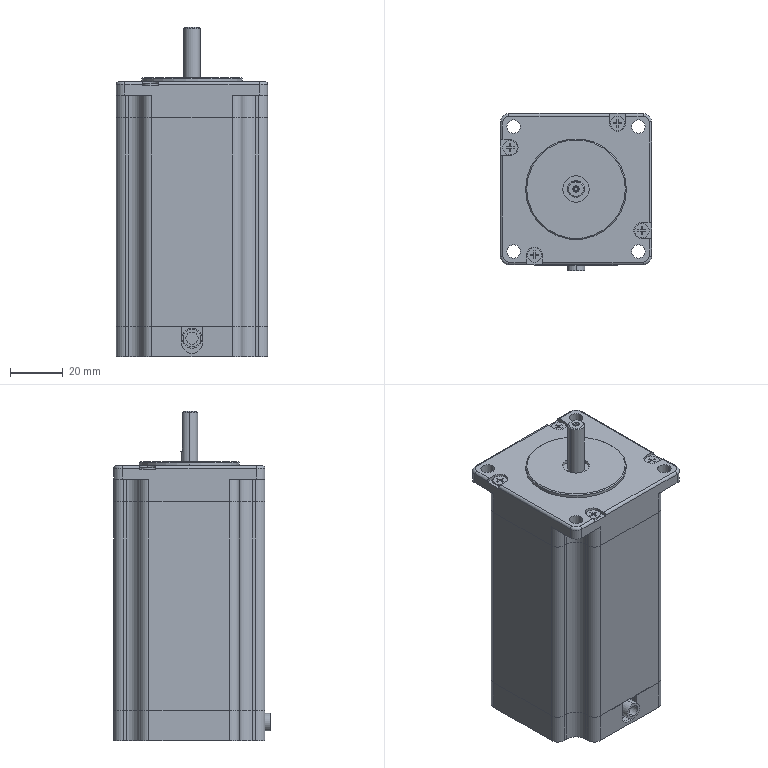Part | SolidWorks | features BaseBody 10 | 10 solids | 292 faces | box 57.2 x 59.232 x 124.486 mm | volume 303415 mm3 | plane 142 | cylinder 117 | cone 17 | spline 12 | torus 4 | commonest cylinder face diameters 3 x28 7.12 x24 9.96 x12 2 x8 5.1 x8 5.5 x8